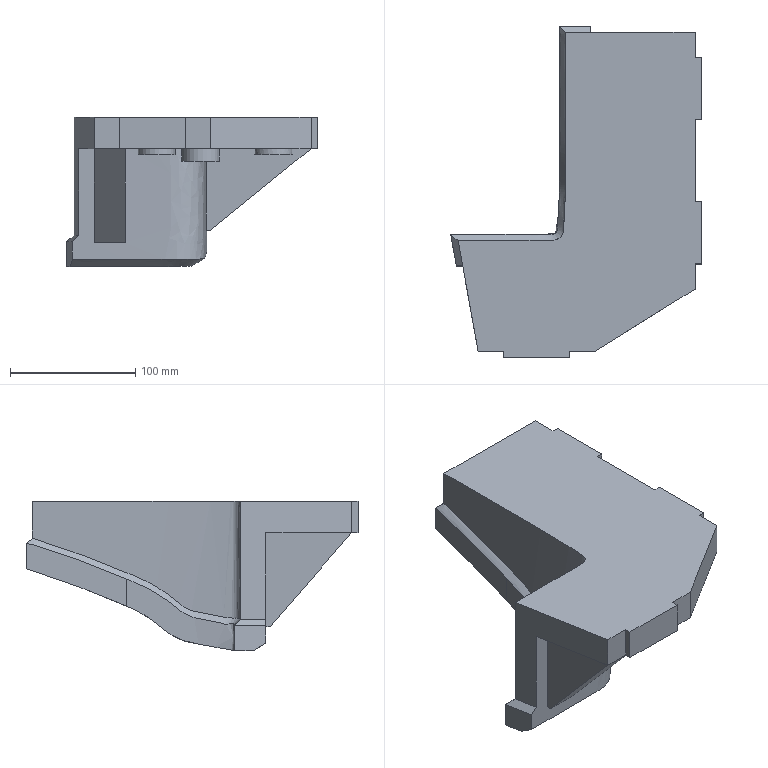Part | NX | features solid 2 | 1 solid | 50 faces | box 200.012 x 265 x 119.195 mm | volume 1380229 mm3 | plane 38 | spline 7 | cylinder 5 | commonest cylinder face diameters 30 x5